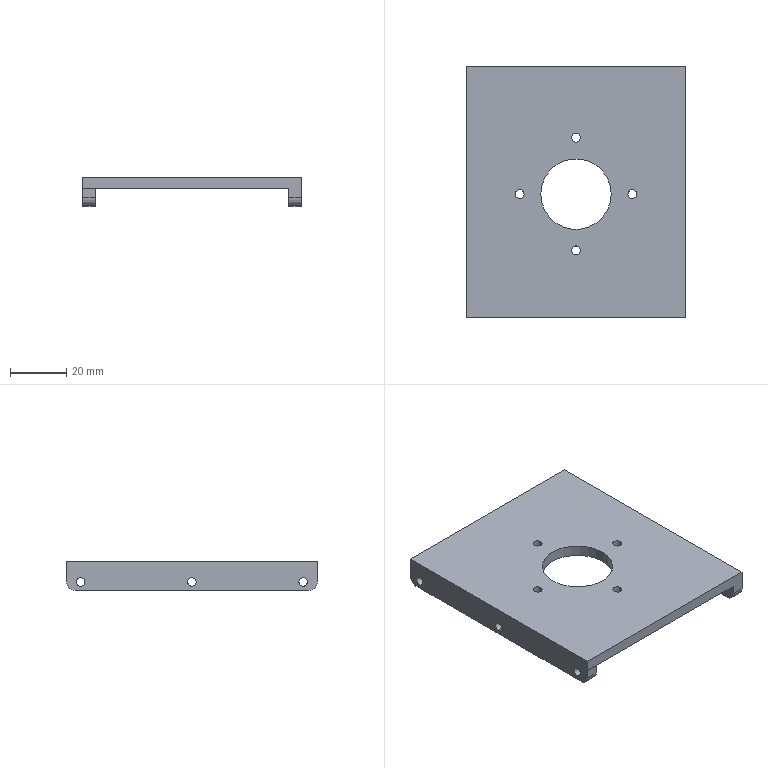Part | NX | features BREP 1 | 1 solid | 37 faces | box 77.6 x 88.919 x 10.2 mm | volume 30243 mm3 | cylinder 26 | plane 11 | commonest cylinder face diameters 3 x12 3.2 x8 6 x4 25 x2
STEP:
#1=CARTESIAN_POINT('',(1.788,32.303,2.5));
#2=VERTEX_POINT('',#1);
#3=CARTESIAN_POINT('',(-1.412,32.303,2.5));
#4=VERTEX_POINT('',#3);
#5=CARTESIAN_POINT('',(0.1876,32.303,2.5));
#6=DIRECTION('',(0.,0.,-1.));
#7=DIRECTION('',(-1.,0.,0.));
#8=AXIS2_PLACEMENT_3D('',#5,#6,#7);
#9=CIRCLE('',#8,1.6);
#10=EDGE_CURVE('',#2,#4,#9,.T.);
#11=ORIENTED_EDGE('',*,*,#10,.F.);
#12=CARTESIAN_POINT('',(1.788,32.303,-1.5));
#13=VERTEX_POINT('',#12);
#14=CARTESIAN_POINT('',(1.788,32.303,2.5));
#15=DIRECTION('',(0.,0.,-1.));
#16=VECTOR('',#15,1000.);
#17=LINE('',#14,#16);
#18=EDGE_CURVE('',#13,#2,#17,.F.);
#19=ORIENTED_EDGE('',*,*,#18,.F.);
#20=CARTESIAN_POINT('',(-1.412,32.303,-1.5));
#21=VERTEX_POINT('',#20);
#22=CARTESIAN_POINT('',(0.1876,32.303,-1.5));
#23=DIRECTION('',(0.,0.,-1.));
#24=DIRECTION('',(-1.,0.,0.));
#25=AXIS2_PLACEMENT_3D('',#22,#23,#24);
#26=CIRCLE('',#25,1.6);
#27=EDGE_CURVE('',#13,#21,#26,.T.);
#28=ORIENTED_EDGE('',*,*,#27,.T.);
#29=CARTESIAN_POINT('',(-1.412,32.303,2.5));
#30=DIRECTION('',(0.,0.,-1.));
#31=VECTOR('',#30,1000.);
#32=LINE('',#29,#31);
#33=EDGE_CURVE('',#21,#4,#32,.F.);
#34=ORIENTED_EDGE('',*,*,#33,.T.);
#35=EDGE_LOOP('',(#11,#19,#28,#34));
#36=FACE_BOUND('',#35,.T.);
#37=CARTESIAN_POINT('',(0.1876,32.303,2.5));
#38=DIRECTION('',(0.,0.,-1.));
#39=DIRECTION('',(1.,0.,0.));
#40=AXIS2_PLACEMENT_3D('',#37,#38,#39);
#41=CYLINDRICAL_SURFACE('',#40,1.6);
#42=ADVANCED_FACE('',(#36),#41,.F.);
#43=CARTESIAN_POINT('',(-18.212,52.303,2.5));
#44=VERTEX_POINT('',#43);
#45=CARTESIAN_POINT('',(-21.412,52.303,2.5));
#46=VERTEX_POINT('',#45);
#47=CARTESIAN_POINT('',(-19.812,52.303,2.5));
#48=DIRECTION('',(0.,0.,-1.));
#49=DIRECTION('',(-1.,0.,0.));
#50=AXIS2_PLACEMENT_3D('',#47,#48,#49);
#51=CIRCLE('',#50,1.6);
#52=EDGE_CURVE('',#44,#46,#51,.T.);
#53=ORIENTED_EDGE('',*,*,#52,.F.);
#54=CARTESIAN_POINT('',(-18.212,52.303,-1.5));
#55=VERTEX_POINT('',#54);
#56=CARTESIAN_POINT('',(-18.212,52.303,2.5));
#57=DIRECTION('',(0.,0.,-1.));
#58=VECTOR('',#57,1000.);
#59=LINE('',#56,#58);
#60=EDGE_CURVE('',#55,#44,#59,.F.);
#61=ORIENTED_EDGE('',*,*,#60,.F.);
#62=CARTESIAN_POINT('',(-21.412,52.303,-1.5));
#63=VERTEX_POINT('',#62);
#64=CARTESIAN_POINT('',(-19.812,52.303,-1.5));
#65=DIRECTION('',(0.,0.,-1.));
#66=DIRECTION('',(-1.,0.,0.));
#67=AXIS2_PLACEMENT_3D('',#64,#65,#66);
#68=CIRCLE('',#67,1.6);
#69=EDGE_CURVE('',#55,#63,#68,.T.);
#70=ORIENTED_EDGE('',*,*,#69,.T.);
#71=CARTESIAN_POINT('',(-21.412,52.303,2.5));
#72=DIRECTION('',(0.,0.,-1.));
#73=VECTOR('',#72,1000.);
#74=LINE('',#71,#73);
#75=EDGE_CURVE('',#63,#46,#74,.F.);
#76=ORIENTED_EDGE('',*,*,#75,.T.);
#77=EDGE_LOOP('',(#53,#61,#70,#76));
#78=FACE_BOUND('',#77,.T.);
#79=CARTESIAN_POINT('',(-19.812,52.303,2.5));
#80=DIRECTION('',(0.,0.,-1.));
#81=DIRECTION('',(1.,0.,0.));
#82=AXIS2_PLACEMENT_3D('',#79,#80,#81);
#83=CYLINDRICAL_SURFACE('',#82,1.6);
#84=ADVANCED_FACE('',(#78),#83,.F.);
#85=CARTESIAN_POINT('',(1.788,72.303,2.5));
#86=VERTEX_POINT('',#85);
#87=CARTESIAN_POINT('',(-1.412,72.303,2.5));
#88=VERTEX_POINT('',#87);
#89=CARTESIAN_POINT('',(0.1876,72.303,2.5));
#90=DIRECTION('',(0.,0.,-1.));
#91=DIRECTION('',(-1.,0.,0.));
#92=AXIS2_PLACEMENT_3D('',#89,#90,#91);
#93=CIRCLE('',#92,1.6);
#94=EDGE_CURVE('',#86,#88,#93,.T.);
#95=ORIENTED_EDGE('',*,*,#94,.F.);
#96=CARTESIAN_POINT('',(1.788,72.303,-1.5));
#97=VERTEX_POINT('',#96);
#98=CARTESIAN_POINT('',(1.788,72.303,2.5));
#99=DIRECTION('',(0.,0.,-1.));
#100=VECTOR('',#99,1000.);
#101=LINE('',#98,#100);
#102=EDGE_CURVE('',#97,#86,#101,.F.);
#103=ORIENTED_EDGE('',*,*,#102,.F.);
#104=CARTESIAN_POINT('',(-1.412,72.303,-1.5));
#105=VERTEX_POINT('',#104);
#106=CARTESIAN_POINT('',(0.1876,72.303,-1.5));
#107=DIRECTION('',(0.,0.,-1.));
#108=DIRECTION('',(-1.,0.,0.));
#109=AXIS2_PLACEMENT_3D('',#106,#107,#108);
#110=CIRCLE('',#109,1.6);
#111=EDGE_CURVE('',#97,#105,#110,.T.);
#112=ORIENTED_EDGE('',*,*,#111,.T.);
#113=CARTESIAN_POINT('',(-1.412,72.303,2.5));
#114=DIRECTION('',(0.,0.,-1.));
#115=VECTOR('',#114,1000.);
#116=LINE('',#113,#115);
#117=EDGE_CURVE('',#105,#88,#116,.F.);
#118=ORIENTED_EDGE('',*,*,#117,.T.);
#119=EDGE_LOOP('',(#95,#103,#112,#118));
#120=FACE_BOUND('',#119,.T.);
#121=CARTESIAN_POINT('',(0.1876,72.303,2.5));
#122=DIRECTION('',(0.,0.,-1.));
#123=DIRECTION('',(1.,0.,0.));
#124=AXIS2_PLACEMENT_3D('',#121,#122,#123);
#125=CYLINDRICAL_SURFACE('',#124,1.6);
#126=ADVANCED_FACE('',(#120),#125,.F.);
#127=CARTESIAN_POINT('',(21.788,52.303,2.5));
#128=VERTEX_POINT('',#127);
#129=CARTESIAN_POINT('',(18.588,52.303,2.5));
#130=VERTEX_POINT('',#129);
#131=CARTESIAN_POINT('',(20.188,52.303,2.5));
#132=DIRECTION('',(0.,0.,-1.));
#133=DIRECTION('',(-1.,0.,0.));
#134=AXIS2_PLACEMENT_3D('',#131,#132,#133);
#135=CIRCLE('',#134,1.6);
#136=EDGE_CURVE('',#128,#130,#135,.T.);
#137=ORIENTED_EDGE('',*,*,#136,.F.);
#138=CARTESIAN_POINT('',(21.788,52.303,-1.5));
#139=VERTEX_POINT('',#138);
#140=CARTESIAN_POINT('',(21.788,52.303,2.5));
#141=DIRECTION('',(0.,0.,-1.));
#142=VECTOR('',#141,1000.);
#143=LINE('',#140,#142);
#144=EDGE_CURVE('',#139,#128,#143,.F.);
#145=ORIENTED_EDGE('',*,*,#144,.F.);
#146=CARTESIAN_POINT('',(18.588,52.303,-1.5));
#147=VERTEX_POINT('',#146);
#148=CARTESIAN_POINT('',(20.188,52.303,-1.5));
#149=DIRECTION('',(0.,0.,-1.));
#150=DIRECTION('',(-1.,0.,0.));
#151=AXIS2_PLACEMENT_3D('',#148,#149,#150);
#152=CIRCLE('',#151,1.6);
#153=EDGE_CURVE('',#139,#147,#152,.T.);
#154=ORIENTED_EDGE('',*,*,#153,.T.);
#155=CARTESIAN_POINT('',(18.588,52.303,2.5));
#156=DIRECTION('',(0.,0.,-1.));
#157=VECTOR('',#156,1000.);
#158=LINE('',#155,#157);
#159=EDGE_CURVE('',#147,#130,#158,.F.);
#160=ORIENTED_EDGE('',*,*,#159,.T.);
#161=EDGE_LOOP('',(#137,#145,#154,#160));
#162=FACE_BOUND('',#161,.T.);
#163=CARTESIAN_POINT('',(20.188,52.303,2.5));
#164=DIRECTION('',(0.,0.,-1.));
#165=DIRECTION('',(1.,0.,0.));
#166=AXIS2_PLACEMENT_3D('',#163,#164,#165);
#167=CYLINDRICAL_SURFACE('',#166,1.6);
#168=ADVANCED_FACE('',(#162),#167,.F.);
#169=CARTESIAN_POINT('',(12.688,52.303,2.5));
#170=VERTEX_POINT('',#169);
#171=CARTESIAN_POINT('',(-12.312,52.303,2.5));
#172=VERTEX_POINT('',#171);
#173=CARTESIAN_POINT('',(0.1876,52.303,2.5));
#174=DIRECTION('',(0.,0.,-1.));
#175=DIRECTION('',(-1.,0.,0.));
#176=AXIS2_PLACEMENT_3D('',#173,#174,#175);
#177=CIRCLE('',#176,12.5);
#178=EDGE_CURVE('',#170,#172,#177,.T.);
#179=ORIENTED_EDGE('',*,*,#178,.F.);
#180=CARTESIAN_POINT('',(12.688,52.303,-1.5));
#181=VERTEX_POINT('',#180);
#182=CARTESIAN_POINT('',(12.688,52.303,2.5));
#183=DIRECTION('',(0.,0.,-1.));
#184=VECTOR('',#183,1000.);
#185=LINE('',#182,#184);
#186=EDGE_CURVE('',#181,#170,#185,.F.);
#187=ORIENTED_EDGE('',*,*,#186,.F.);
#188=CARTESIAN_POINT('',(-12.312,52.303,-1.5));
#189=VERTEX_POINT('',#188);
#190=CARTESIAN_POINT('',(0.1876,52.303,-1.5));
#191=DIRECTION('',(0.,0.,-1.));
#192=DIRECTION('',(-1.,0.,0.));
#193=AXIS2_PLACEMENT_3D('',#190,#191,#192);
#194=CIRCLE('',#193,12.5);
#195=EDGE_CURVE('',#181,#189,#194,.T.);
#196=ORIENTED_EDGE('',*,*,#195,.T.);
#197=CARTESIAN_POINT('',(-12.312,52.303,2.5));
#198=DIRECTION('',(0.,0.,-1.));
#199=VECTOR('',#198,1000.);
#200=LINE('',#197,#199);
#201=EDGE_CURVE('',#189,#172,#200,.F.);
#202=ORIENTED_EDGE('',*,*,#201,.T.);
#203=EDGE_LOOP('',(#179,#187,#196,#202));
#204=FACE_BOUND('',#203,.T.);
#205=CARTESIAN_POINT('',(0.1876,52.303,2.5));
#206=DIRECTION('',(0.,0.,-1.));
#207=DIRECTION('',(1.,0.,0.));
#208=AXIS2_PLACEMENT_3D('',#205,#206,#207);
#209=CYLINDRICAL_SURFACE('',#208,12.5);
#210=ADVANCED_FACE('',(#204),#209,.F.);
#211=CARTESIAN_POINT('',(38.988,92.505,-6.2));
#212=VERTEX_POINT('',#211);
#213=CARTESIAN_POINT('',(38.988,92.505,-3.2));
#214=VERTEX_POINT('',#213);
#215=CARTESIAN_POINT('',(38.988,92.505,-4.7));
#216=DIRECTION('',(-1.,0.,0.));
#217=DIRECTION('',(0.,-1.,0.));
#218=AXIS2_PLACEMENT_3D('',#215,#216,#217);
#219=CIRCLE('',#218,1.5);
#220=EDGE_CURVE('',#212,#214,#219,.T.);
#221=ORIENTED_EDGE('',*,*,#220,.F.);
#222=CARTESIAN_POINT('',(34.488,92.505,-6.2));
#223=VERTEX_POINT('',#222);
#224=CARTESIAN_POINT('',(59.388,92.505,-6.2));
#225=DIRECTION('',(-1.,0.,0.));
#226=VECTOR('',#225,1000.);
#227=LINE('',#224,#226);
#228=EDGE_CURVE('',#212,#223,#227,.T.);
#229=ORIENTED_EDGE('',*,*,#228,.T.);
#230=CARTESIAN_POINT('',(34.488,92.505,-3.2));
#231=VERTEX_POINT('',#230);
#232=CARTESIAN_POINT('',(34.488,92.505,-4.7));
#233=DIRECTION('',(1.,0.,0.));
#234=DIRECTION('',(0.,0.,-1.));
#235=AXIS2_PLACEMENT_3D('',#232,#233,#234);
#236=CIRCLE('',#235,1.5);
#237=EDGE_CURVE('',#231,#223,#236,.T.);
#238=ORIENTED_EDGE('',*,*,#237,.F.);
#239=CARTESIAN_POINT('',(59.388,92.505,-3.2));
#240=DIRECTION('',(-1.,0.,0.));
#241=VECTOR('',#240,1000.);
#242=LINE('',#239,#241);
#243=EDGE_CURVE('',#214,#231,#242,.T.);
#244=ORIENTED_EDGE('',*,*,#243,.F.);
#245=EDGE_LOOP('',(#221,#229,#238,#244));
#246=FACE_BOUND('',#245,.T.);
#247=CARTESIAN_POINT('',(59.388,92.505,-4.7));
#248=DIRECTION('',(-1.,0.,0.));
#249=DIRECTION('',(0.,0.,-1.));
#250=AXIS2_PLACEMENT_3D('',#247,#248,#249);
#251=CYLINDRICAL_SURFACE('',#250,1.5);
#252=ADVANCED_FACE('',(#246),#251,.F.);
#253=CARTESIAN_POINT('',(-34.112,92.505,-6.2));
#254=VERTEX_POINT('',#253);
#255=CARTESIAN_POINT('',(-34.112,92.505,-3.2));
#256=VERTEX_POINT('',#255);
#257=CARTESIAN_POINT('',(-34.112,92.505,-4.7));
#258=DIRECTION('',(-1.,0.,0.));
#259=DIRECTION('',(0.,0.,1.));
#260=AXIS2_PLACEMENT_3D('',#257,#258,#259);
#261=CIRCLE('',#260,1.5);
#262=EDGE_CURVE('',#254,#256,#261,.T.);
#263=ORIENTED_EDGE('',*,*,#262,.F.);
#264=CARTESIAN_POINT('',(-38.612,92.505,-6.2));
#265=VERTEX_POINT('',#264);
#266=CARTESIAN_POINT('',(-18.612,92.505,-6.2));
#267=DIRECTION('',(-1.,0.,0.));
#268=VECTOR('',#267,1000.);
#269=LINE('',#266,#268);
#270=EDGE_CURVE('',#254,#265,#269,.T.);
#271=ORIENTED_EDGE('',*,*,#270,.T.);
#272=CARTESIAN_POINT('',(-38.612,92.505,-3.2));
#273=VERTEX_POINT('',#272);
#274=CARTESIAN_POINT('',(-38.612,92.505,-4.7));
#275=DIRECTION('',(-1.,0.,0.));
#276=DIRECTION('',(0.,0.,1.));
#277=AXIS2_PLACEMENT_3D('',#274,#275,#276);
#278=CIRCLE('',#277,1.5);
#279=EDGE_CURVE('',#265,#273,#278,.T.);
#280=ORIENTED_EDGE('',*,*,#279,.T.);
#281=CARTESIAN_POINT('',(-18.612,92.505,-3.2));
#282=DIRECTION('',(-1.,0.,0.));
#283=VECTOR('',#282,1000.);
#284=LINE('',#281,#283);
#285=EDGE_CURVE('',#256,#273,#284,.T.);
#286=ORIENTED_EDGE('',*,*,#285,.F.);
#287=EDGE_LOOP('',(#263,#271,#280,#286));
#288=FACE_BOUND('',#287,.T.);
#289=CARTESIAN_POINT('',(-18.612,92.505,-4.7));
#290=DIRECTION('',(-1.,0.,0.));
#291=DIRECTION('',(0.,0.,-1.));
#292=AXIS2_PLACEMENT_3D('',#289,#290,#291);
#293=CYLINDRICAL_SURFACE('',#292,1.5);
#294=ADVANCED_FACE('',(#288),#293,.F.);
#295=CARTESIAN_POINT('',(-34.112,13.621,-6.2));
#296=VERTEX_POINT('',#295);
#297=CARTESIAN_POINT('',(-34.112,13.621,-3.2));
#298=VERTEX_POINT('',#297);
#299=CARTESIAN_POINT('',(-34.112,13.621,-4.7));
#300=DIRECTION('',(-1.,0.,0.));
#301=DIRECTION('',(0.,0.,1.));
#302=AXIS2_PLACEMENT_3D('',#299,#300,#301);
#303=CIRCLE('',#302,1.5);
#304=EDGE_CURVE('',#296,#298,#303,.T.);
#305=ORIENTED_EDGE('',*,*,#304,.F.);
#306=CARTESIAN_POINT('',(-38.612,13.621,-6.2));
#307=VERTEX_POINT('',#306);
#308=CARTESIAN_POINT('',(-18.612,13.621,-6.2));
#309=DIRECTION('',(-1.,0.,0.));
#310=VECTOR('',#309,1000.);
#311=LINE('',#308,#310);
#312=EDGE_CURVE('',#296,#307,#311,.T.);
#313=ORIENTED_EDGE('',*,*,#312,.T.);
#314=CARTESIAN_POINT('',(-38.612,13.621,-3.2));
#315=VERTEX_POINT('',#314);
#316=CARTESIAN_POINT('',(-38.612,13.621,-4.7));
#317=DIRECTION('',(-1.,0.,0.));
#318=DIRECTION('',(0.,0.,1.));
#319=AXIS2_PLACEMENT_3D('',#316,#317,#318);
#320=CIRCLE('',#319,1.5);
#321=EDGE_CURVE('',#307,#315,#320,.T.);
#322=ORIENTED_EDGE('',*,*,#321,.T.);
#323=CARTESIAN_POINT('',(-18.612,13.621,-3.2));
#324=DIRECTION('',(-1.,0.,0.));
#325=VECTOR('',#324,1000.);
#326=LINE('',#323,#325);
#327=EDGE_CURVE('',#298,#315,#326,.T.);
#328=ORIENTED_EDGE('',*,*,#327,.F.);
#329=EDGE_LOOP('',(#305,#313,#322,#328));
#330=FACE_BOUND('',#329,.T.);
#331=CARTESIAN_POINT('',(-18.612,13.621,-4.7));
#332=DIRECTION('',(-1.,0.,0.));
#333=DIRECTION('',(0.,0.,-1.));
#334=AXIS2_PLACEMENT_3D('',#331,#332,#333);
#335=CYLINDRICAL_SURFACE('',#334,1.5);
#336=ADVANCED_FACE('',(#330),#335,.F.);
#337=CARTESIAN_POINT('',(-34.112,53.063,-6.2));
#338=VERTEX_POINT('',#337);
#339=CARTESIAN_POINT('',(-34.112,53.063,-3.2));
#340=VERTEX_POINT('',#339);
#341=CARTESIAN_POINT('',(-34.112,53.063,-4.7));
#342=DIRECTION('',(-1.,0.,0.));
#343=DIRECTION('',(0.,0.,1.));
#344=AXIS2_PLACEMENT_3D('',#341,#342,#343);
#345=CIRCLE('',#344,1.5);
#346=EDGE_CURVE('',#338,#340,#345,.T.);
#347=ORIENTED_EDGE('',*,*,#346,.F.);
#348=CARTESIAN_POINT('',(-38.612,53.063,-6.2));
#349=VERTEX_POINT('',#348);
#350=CARTESIAN_POINT('',(-18.612,53.063,-6.2));
#351=DIRECTION('',(-1.,0.,0.));
#352=VECTOR('',#351,1000.);
#353=LINE('',#350,#352);
#354=EDGE_CURVE('',#338,#349,#353,.T.);
#355=ORIENTED_EDGE('',*,*,#354,.T.);
#356=CARTESIAN_POINT('',(-38.612,53.063,-3.2));
#357=VERTEX_POINT('',#356);
#358=CARTESIAN_POINT('',(-38.612,53.063,-4.7));
#359=DIRECTION('',(-1.,0.,0.));
#360=DIRECTION('',(0.,0.,1.));
#361=AXIS2_PLACEMENT_3D('',#358,#359,#360);
#362=CIRCLE('',#361,1.5);
#363=EDGE_CURVE('',#349,#357,#362,.T.);
#364=ORIENTED_EDGE('',*,*,#363,.T.);
#365=CARTESIAN_POINT('',(-18.612,53.063,-3.2));
#366=DIRECTION('',(-1.,0.,0.));
#367=VECTOR('',#366,1000.);
#368=LINE('',#365,#367);
#369=EDGE_CURVE('',#340,#357,#368,.T.);
#370=ORIENTED_EDGE('',*,*,#369,.F.);
#371=EDGE_LOOP('',(#347,#355,#364,#370));
#372=FACE_BOUND('',#371,.T.);
#373=CARTESIAN_POINT('',(-18.612,53.063,-4.7));
#374=DIRECTION('',(-1.,0.,0.));
#375=DIRECTION('',(0.,0.,-1.));
#376=AXIS2_PLACEMENT_3D('',#373,#374,#375);
#377=CYLINDRICAL_SURFACE('',#376,1.5);
#378=ADVANCED_FACE('',(#372),#377,.F.);
#379=CARTESIAN_POINT('',(34.488,12.121,-4.7));
#380=VERTEX_POINT('',#379);
#381=CARTESIAN_POINT('',(34.488,15.121,-4.7));
#382=VERTEX_POINT('',#381);
#383=CARTESIAN_POINT('',(34.488,13.621,-4.7));
#384=DIRECTION('',(1.,0.,0.));
#385=DIRECTION('',(0.,0.,-1.));
#386=AXIS2_PLACEMENT_3D('',#383,#384,#385);
#387=CIRCLE('',#386,1.5);
#388=EDGE_CURVE('',#380,#382,#387,.T.);
#389=ORIENTED_EDGE('',*,*,#388,.F.);
#390=CARTESIAN_POINT('',(38.988,12.121,-4.7));
#391=VERTEX_POINT('',#390);
#392=CARTESIAN_POINT('',(28.988,12.121,-4.7));
#393=DIRECTION('',(1.,0.,0.));
#394=VECTOR('',#393,1000.);
#395=LINE('',#392,#394);
#396=EDGE_CURVE('',#380,#391,#395,.T.);
#397=ORIENTED_EDGE('',*,*,#396,.T.);
#398=CARTESIAN_POINT('',(38.988,15.121,-4.7));
#399=VERTEX_POINT('',#398);
#400=CARTESIAN_POINT('',(38.988,13.621,-4.7));
#401=DIRECTION('',(-1.,0.,0.));
#402=DIRECTION('',(0.,-1.,0.));
#403=AXIS2_PLACEMENT_3D('',#400,#401,#402);
#404=CIRCLE('',#403,1.5);
#405=EDGE_CURVE('',#399,#391,#404,.T.);
#406=ORIENTED_EDGE('',*,*,#405,.F.);
#407=CARTESIAN_POINT('',(28.988,15.121,-4.7));
#408=DIRECTION('',(1.,0.,0.));
#409=VECTOR('',#408,1000.);
#410=LINE('',#407,#409);
#411=EDGE_CURVE('',#382,#399,#410,.T.);
#412=ORIENTED_EDGE('',*,*,#411,.F.);
#413=EDGE_LOOP('',(#389,#397,#406,#412));
#414=FACE_BOUND('',#413,.T.);
#415=CARTESIAN_POINT('',(28.988,13.621,-4.7));
#416=DIRECTION('',(1.,0.,0.));
#417=DIRECTION('',(0.,-1.,0.));
#418=AXIS2_PLACEMENT_3D('',#415,#416,#417);
#419=CYLINDRICAL_SURFACE('',#418,1.5);
#420=ADVANCED_FACE('',(#414),#419,.F.);
#421=CARTESIAN_POINT('',(34.488,51.563,-4.7));
#422=VERTEX_POINT('',#421);
#423=CARTESIAN_POINT('',(34.488,54.563,-4.7));
#424=VERTEX_POINT('',#423);
#425=CARTESIAN_POINT('',(34.488,53.063,-4.7));
#426=DIRECTION('',(1.,0.,0.));
#427=DIRECTION('',(0.,0.,-1.));
#428=AXIS2_PLACEMENT_3D('',#425,#426,#427);
#429=CIRCLE('',#428,1.5);
#430=EDGE_CURVE('',#422,#424,#429,.T.);
#431=ORIENTED_EDGE('',*,*,#430,.F.);
#432=CARTESIAN_POINT('',(38.988,51.563,-4.7));
#433=VERTEX_POINT('',#432);
#434=CARTESIAN_POINT('',(28.988,51.563,-4.7));
#435=DIRECTION('',(1.,0.,0.));
#436=VECTOR('',#435,1000.);
#437=LINE('',#434,#436);
#438=EDGE_CURVE('',#422,#433,#437,.T.);
#439=ORIENTED_EDGE('',*,*,#438,.T.);
#440=CARTESIAN_POINT('',(38.988,54.563,-4.7));
#441=VERTEX_POINT('',#440);
#442=CARTESIAN_POINT('',(38.988,53.063,-4.7));
#443=DIRECTION('',(-1.,0.,0.));
#444=DIRECTION('',(0.,-1.,0.));
#445=AXIS2_PLACEMENT_3D('',#442,#443,#444);
#446=CIRCLE('',#445,1.5);
#447=EDGE_CURVE('',#441,#433,#446,.T.);
#448=ORIENTED_EDGE('',*,*,#447,.F.);
#449=CARTESIAN_POINT('',(28.988,54.563,-4.7));
#450=DIRECTION('',(1.,0.,0.));
#451=VECTOR('',#450,1000.);
#452=LINE('',#449,#451);
#453=EDGE_CURVE('',#424,#441,#452,.T.);
#454=ORIENTED_EDGE('',*,*,#453,.F.);
#455=EDGE_LOOP('',(#431,#439,#448,#454));
#456=FACE_BOUND('',#455,.T.);
#457=CARTESIAN_POINT('',(28.988,53.063,-4.7));
#458=DIRECTION('',(1.,0.,0.));
#459=DIRECTION('',(0.,-1.,0.));
#460=AXIS2_PLACEMENT_3D('',#457,#458,#459);
#461=CYLINDRICAL_SURFACE('',#460,1.5);
#462=ADVANCED_FACE('',(#456),#461,.F.);
#463=CARTESIAN_POINT('',(38.988,97.505,-4.7));
#464=VERTEX_POINT('',#463);
#465=CARTESIAN_POINT('',(34.488,97.505,-4.7));
#466=VERTEX_POINT('',#465);
#467=CARTESIAN_POINT('',(40.988,97.505,-4.7));
#468=DIRECTION('',(-1.,0.,0.));
#469=VECTOR('',#468,1000.);
#470=LINE('',#467,#469);
#471=EDGE_CURVE('',#464,#466,#470,.T.);
#472=ORIENTED_EDGE('',*,*,#471,.F.);
#473=CARTESIAN_POINT('',(38.988,94.505,-7.7));
#474=VERTEX_POINT('',#473);
#475=CARTESIAN_POINT('',(38.988,94.505,-4.7));
#476=DIRECTION('',(-1.,0.,0.));
#477=DIRECTION('',(0.,-1.,0.));
#478=AXIS2_PLACEMENT_3D('',#475,#476,#477);
#479=CIRCLE('',#478,3.);
#480=EDGE_CURVE('',#464,#474,#479,.T.);
#481=ORIENTED_EDGE('',*,*,#480,.T.);
#482=CARTESIAN_POINT('',(34.488,94.505,-7.7));
#483=VERTEX_POINT('',#482);
#484=CARTESIAN_POINT('',(-27.612,94.505,-7.7));
#485=DIRECTION('',(1.,0.,0.));
#486=VECTOR('',#485,1000.);
#487=LINE('',#484,#486);
#488=EDGE_CURVE('',#483,#474,#487,.T.);
#489=ORIENTED_EDGE('',*,*,#488,.F.);
#490=CARTESIAN_POINT('',(34.488,94.505,-4.7));
#491=DIRECTION('',(-1.,0.,0.));
#492=DIRECTION('',(0.,0.,-1.));
#493=AXIS2_PLACEMENT_3D('',#490,#491,#492);
#494=CIRCLE('',#493,3.);
#495=EDGE_CURVE('',#466,#483,#494,.T.);
#496=ORIENTED_EDGE('',*,*,#495,.F.);
#497=EDGE_LOOP('',(#472,#481,#489,#496));
#498=FACE_BOUND('',#497,.T.);
#499=CARTESIAN_POINT('',(40.988,94.505,-4.7));
#500=DIRECTION('',(-1.,0.,0.));
#501=DIRECTION('',(0.,0.,-1.));
#502=AXIS2_PLACEMENT_3D('',#499,#500,#501);
#503=CYLINDRICAL_SURFACE('',#502,3.);
#504=ADVANCED_FACE('',(#498),#503,.T.);
#505=ORIENTED_EDGE('',*,*,#438,.F.);
#506=CARTESIAN_POINT('',(34.488,53.063,-4.7));
#507=DIRECTION('',(1.,0.,0.));
#508=DIRECTION('',(0.,0.,-1.));
#509=AXIS2_PLACEMENT_3D('',#506,#507,#508);
#510=CIRCLE('',#509,1.5);
#511=EDGE_CURVE('',#424,#422,#510,.T.);
#512=ORIENTED_EDGE('',*,*,#511,.F.);
#513=ORIENTED_EDGE('',*,*,#453,.T.);
#514=CARTESIAN_POINT('',(38.988,53.063,-4.7));
#515=DIRECTION('',(-1.,0.,0.));
#516=DIRECTION('',(0.,-1.,0.));
#517=AXIS2_PLACEMENT_3D('',#514,#515,#516);
#518=CIRCLE('',#517,1.5);
#519=EDGE_CURVE('',#433,#441,#518,.T.);
#520=ORIENTED_EDGE('',*,*,#519,.F.);
#521=EDGE_LOOP('',(#505,#512,#513,#520));
#522=FACE_BOUND('',#521,.T.);
#523=CARTESIAN_POINT('',(28.988,53.063,-4.7));
#524=DIRECTION('',(1.,0.,0.));
#525=DIRECTION('',(0.,-1.,0.));
#526=AXIS2_PLACEMENT_3D('',#523,#524,#525);
#527=CYLINDRICAL_SURFACE('',#526,1.5);
#528=ADVANCED_FACE('',(#522),#527,.F.);
#529=ORIENTED_EDGE('',*,*,#396,.F.);
#530=CARTESIAN_POINT('',(34.488,13.621,-4.7));
#531=DIRECTION('',(1.,0.,0.));
#532=DIRECTION('',(0.,0.,-1.));
#533=AXIS2_PLACEMENT_3D('',#530,#531,#532);
#534=CIRCLE('',#533,1.5);
#535=EDGE_CURVE('',#382,#380,#534,.T.);
#536=ORIENTED_EDGE('',*,*,#535,.F.);
#537=ORIENTED_EDGE('',*,*,#411,.T.);
#538=CARTESIAN_POINT('',(38.988,13.621,-4.7));
#539=DIRECTION('',(-1.,0.,0.));
#540=DIRECTION('',(0.,-1.,0.));
#541=AXIS2_PLACEMENT_3D('',#538,#539,#540);
#542=CIRCLE('',#541,1.5);
#543=EDGE_CURVE('',#391,#399,#542,.T.);
#544=ORIENTED_EDGE('',*,*,#543,.F.);
#545=EDGE_LOOP('',(#529,#536,#537,#544));
#546=FACE_BOUND('',#545,.T.);
#547=CARTESIAN_POINT('',(28.988,13.621,-4.7));
#548=DIRECTION('',(1.,0.,0.));
#549=DIRECTION('',(0.,-1.,0.));
#550=AXIS2_PLACEMENT_3D('',#547,#548,#549);
#551=CYLINDRICAL_SURFACE('',#550,1.5);
#552=ADVANCED_FACE('',(#546),#551,.F.);
#553=CARTESIAN_POINT('',(38.988,11.586,-7.7));
#554=VERTEX_POINT('',#553);
#555=CARTESIAN_POINT('',(34.488,11.586,-7.7));
#556=VERTEX_POINT('',#555);
#557=CARTESIAN_POINT('',(-27.612,11.586,-7.7));
#558=DIRECTION('',(-1.,0.,0.));
#559=VECTOR('',#558,1000.);
#560=LINE('',#557,#559);
#561=EDGE_CURVE('',#554,#556,#560,.T.);
#562=ORIENTED_EDGE('',*,*,#561,.F.);
#563=CARTESIAN_POINT('',(38.988,8.586,-4.7));
#564=VERTEX_POINT('',#563);
#565=CARTESIAN_POINT('',(38.988,11.586,-4.7));
#566=DIRECTION('',(-1.,0.,0.));
#567=DIRECTION('',(0.,-1.,0.));
#568=AXIS2_PLACEMENT_3D('',#565,#566,#567);
#569=CIRCLE('',#568,3.);
#570=EDGE_CURVE('',#554,#564,#569,.T.);
#571=ORIENTED_EDGE('',*,*,#570,.T.);
#572=CARTESIAN_POINT('',(34.488,8.586,-4.7));
#573=VERTEX_POINT('',#572);
#574=CARTESIAN_POINT('',(40.988,8.586,-4.7));
#575=DIRECTION('',(1.,0.,0.));
#576=VECTOR('',#575,1000.);
#577=LINE('',#574,#576);
#578=EDGE_CURVE('',#573,#564,#577,.T.);
#579=ORIENTED_EDGE('',*,*,#578,.F.);
#580=CARTESIAN_POINT('',(34.488,11.586,-4.7));
#581=DIRECTION('',(-1.,0.,0.));
#582=DIRECTION('',(0.,0.,-1.));
#583=AXIS2_PLACEMENT_3D('',#580,#581,#582);
#584=CIRCLE('',#583,3.);
#585=EDGE_CURVE('',#556,#573,#584,.T.);
#586=ORIENTED_EDGE('',*,*,#585,.F.);
#587=EDGE_LOOP('',(#562,#571,#579,#586));
#588=FACE_BOUND('',#587,.T.);
#589=CARTESIAN_POINT('',(40.988,11.586,-4.7));
#590=DIRECTION('',(1.,0.,0.));
#591=DIRECTION('',(0.,-1.,0.));
#592=AXIS2_PLACEMENT_3D('',#589,#590,#591);
#593=CYLINDRICAL_SURFACE('',#592,3.);
#594=ADVANCED_FACE('',(#588),#593,.T.);
#595=CARTESIAN_POINT('',(-38.612,8.586,-1.5));
#596=VERTEX_POINT('',#595);
#597=CARTESIAN_POINT('',(34.488,8.586,-1.5));
#598=VERTEX_POINT('',#597);
#599=CARTESIAN_POINT('',(40.988,8.586,-1.5));
#600=DIRECTION('',(1.,0.,0.));
#601=VECTOR('',#600,1000.);
#602=LINE('',#599,#601);
#603=EDGE_CURVE('',#596,#598,#602,.T.);
#604=ORIENTED_EDGE('',*,*,#603,.F.);
#605=CARTESIAN_POINT('',(-38.612,8.621,-1.5));
#606=VERTEX_POINT('',#605);
#607=CARTESIAN_POINT('',(-38.612,8.621,-1.5));
#608=DIRECTION('',(0.,-1.,0.));
#609=VECTOR('',#608,1000.);
#610=LINE('',#607,#609);
#611=EDGE_CURVE('',#606,#596,#610,.T.);
#612=ORIENTED_EDGE('',*,*,#611,.F.);
#613=CARTESIAN_POINT('',(-34.112,8.621,-1.5));
#614=VERTEX_POINT('',#613);
#615=CARTESIAN_POINT('',(-38.612,8.621,-1.5));
#616=DIRECTION('',(-1.,0.,0.));
#617=VECTOR('',#616,1000.);
#618=LINE('',#615,#617);
#619=EDGE_CURVE('',#614,#606,#618,.T.);
#620=ORIENTED_EDGE('',*,*,#619,.F.);
#621=CARTESIAN_POINT('',(-34.112,97.505,-1.5));
#622=VERTEX_POINT('',#621);
#623=CARTESIAN_POINT('',(-34.112,97.505,-1.5));
#624=DIRECTION('',(0.,-1.,0.));
#625=VECTOR('',#624,1000.);
#626=LINE('',#623,#625);
#627=EDGE_CURVE('',#622,#614,#626,.T.);
#628=ORIENTED_EDGE('',*,*,#627,.F.);
#629=CARTESIAN_POINT('',(34.488,97.505,-1.5));
#630=VERTEX_POINT('',#629);
#631=CARTESIAN_POINT('',(40.988,97.505,-1.5));
#632=DIRECTION('',(-1.,0.,0.));
#633=VECTOR('',#632,1000.);
#634=LINE('',#631,#633);
#635=EDGE_CURVE('',#630,#622,#634,.T.);
#636=ORIENTED_EDGE('',*,*,#635,.F.);
#637=CARTESIAN_POINT('',(34.488,8.586,-1.5));
#638=DIRECTION('',(0.,1.,0.));
#639=VECTOR('',#638,1000.);
#640=LINE('',#637,#639);
#641=EDGE_CURVE('',#598,#630,#640,.T.);
#642=ORIENTED_EDGE('',*,*,#641,.F.);
#643=EDGE_LOOP('',(#604,#612,#620,#628,#636,#642));
#644=FACE_BOUND('',#643,.T.);
#645=CARTESIAN_POINT('',(0.1876,32.303,-1.5));
#646=DIRECTION('',(0.,0.,-1.));
#647=DIRECTION('',(-1.,0.,0.));
#648=AXIS2_PLACEMENT_3D('',#645,#646,#647);
#649=CIRCLE('',#648,1.6);
#650=EDGE_CURVE('',#21,#13,#649,.T.);
#651=ORIENTED_EDGE('',*,*,#650,.F.);
#652=ORIENTED_EDGE('',*,*,#27,.F.);
#653=EDGE_LOOP('',(#651,#652));
#654=FACE_BOUND('',#653,.T.);
#655=CARTESIAN_POINT('',(-19.812,52.303,-1.5));
#656=DIRECTION('',(0.,0.,-1.));
#657=DIRECTION('',(-1.,0.,0.));
#658=AXIS2_PLACEMENT_3D('',#655,#656,#657);
#659=CIRCLE('',#658,1.6);
#660=EDGE_CURVE('',#63,#55,#659,.T.);
#661=ORIENTED_EDGE('',*,*,#660,.F.);
#662=ORIENTED_EDGE('',*,*,#69,.F.);
#663=EDGE_LOOP('',(#661,#662));
#664=FACE_BOUND('',#663,.T.);
#665=CARTESIAN_POINT('',(0.1876,72.303,-1.5));
#666=DIRECTION('',(0.,0.,-1.));
#667=DIRECTION('',(-1.,0.,0.));
#668=AXIS2_PLACEMENT_3D('',#665,#666,#667);
#669=CIRCLE('',#668,1.6);
#670=EDGE_CURVE('',#105,#97,#669,.T.);
#671=ORIENTED_EDGE('',*,*,#670,.F.);
#672=ORIENTED_EDGE('',*,*,#111,.F.);
#673=EDGE_LOOP('',(#671,#672));
#674=FACE_BOUND('',#673,.T.);
#675=CARTESIAN_POINT('',(20.188,52.303,-1.5));
#676=DIRECTION('',(0.,0.,-1.));
#677=DIRECTION('',(-1.,0.,0.));
#678=AXIS2_PLACEMENT_3D('',#675,#676,#677);
#679=CIRCLE('',#678,1.6);
#680=EDGE_CURVE('',#147,#139,#679,.T.);
#681=ORIENTED_EDGE('',*,*,#680,.F.);
#682=ORIENTED_EDGE('',*,*,#153,.F.);
#683=EDGE_LOOP('',(#681,#682));
#684=FACE_BOUND('',#683,.T.);
#685=CARTESIAN_POINT('',(0.1876,52.303,-1.5));
#686=DIRECTION('',(0.,0.,-1.));
#687=DIRECTION('',(-1.,0.,0.));
#688=AXIS2_PLACEMENT_3D('',#685,#686,#687);
#689=CIRCLE('',#688,12.5);
#690=EDGE_CURVE('',#189,#181,#689,.T.);
#691=ORIENTED_EDGE('',*,*,#690,.F.);
#692=ORIENTED_EDGE('',*,*,#195,.F.);
#693=EDGE_LOOP('',(#691,#692));
#694=FACE_BOUND('',#693,.T.);
#695=CARTESIAN_POINT('',(0.,0.,-1.5));
#696=DIRECTION('',(0.,0.,1.));
#697=DIRECTION('',(-1.,0.,0.));
#698=AXIS2_PLACEMENT_3D('',#695,#696,#697);
#699=PLANE('',#698);
#700=ADVANCED_FACE('',(#644,#654,#664,#674,#684,#694),#699,.F.);
#701=ORIENTED_EDGE('',*,*,#619,.T.);
#702=CARTESIAN_POINT('',(-38.612,8.621,-4.7));
#703=VERTEX_POINT('',#702);
#704=CARTESIAN_POINT('',(-38.612,8.621,-4.7));
#705=DIRECTION('',(0.,0.,1.));
#706=VECTOR('',#705,1000.);
#707=LINE('',#704,#706);
#708=EDGE_CURVE('',#703,#606,#707,.T.);
#709=ORIENTED_EDGE('',*,*,#708,.F.);
#710=CARTESIAN_POINT('',(-34.112,8.621,-4.7));
#711=VERTEX_POINT('',#710);
#712=CARTESIAN_POINT('',(-38.612,8.621,-4.7));
#713=DIRECTION('',(1.,0.,0.));
#714=VECTOR('',#713,1000.);
#715=LINE('',#712,#714);
#716=EDGE_CURVE('',#703,#711,#715,.T.);
#717=ORIENTED_EDGE('',*,*,#716,.T.);
#718=CARTESIAN_POINT('',(-34.112,8.621,-95.698));
#719=DIRECTION('',(0.,0.,1.));
#720=VECTOR('',#719,1000.);
#721=LINE('',#718,#720);
#722=EDGE_CURVE('',#711,#614,#721,.T.);
#723=ORIENTED_EDGE('',*,*,#722,.T.);
#724=EDGE_LOOP('',(#701,#709,#717,#723));
#725=FACE_BOUND('',#724,.T.);
#726=CARTESIAN_POINT('',(-38.612,8.621,-95.698));
#727=DIRECTION('',(0.,1.,0.));
#728=DIRECTION('',(-1.,0.,0.));
#729=AXIS2_PLACEMENT_3D('',#726,#727,#728);
#730=PLANE('',#729);
#731=ADVANCED_FACE('',(#725),#730,.F.);
#732=ORIENTED_EDGE('',*,*,#354,.F.);
#733=CARTESIAN_POINT('',(-34.112,53.063,-4.7));
#734=DIRECTION('',(-1.,0.,0.));
#735=DIRECTION('',(0.,0.,1.));
#736=AXIS2_PLACEMENT_3D('',#733,#734,#735);
#737=CIRCLE('',#736,1.5);
#738=EDGE_CURVE('',#340,#338,#737,.T.);
#739=ORIENTED_EDGE('',*,*,#738,.F.);
#740=ORIENTED_EDGE('',*,*,#369,.T.);
#741=CARTESIAN_POINT('',(-38.612,53.063,-4.7));
#742=DIRECTION('',(-1.,0.,0.));
#743=DIRECTION('',(0.,0.,1.));
#744=AXIS2_PLACEMENT_3D('',#741,#742,#743);
#745=CIRCLE('',#744,1.5);
#746=EDGE_CURVE('',#357,#349,#745,.T.);
#747=ORIENTED_EDGE('',*,*,#746,.T.);
#748=EDGE_LOOP('',(#732,#739,#740,#747));
#749=FACE_BOUND('',#748,.T.);
#750=CARTESIAN_POINT('',(-18.612,53.063,-4.7));
#751=DIRECTION('',(-1.,0.,0.));
#752=DIRECTION('',(0.,0.,-1.));
#753=AXIS2_PLACEMENT_3D('',#750,#751,#752);
#754=CYLINDRICAL_SURFACE('',#753,1.5);
#755=ADVANCED_FACE('',(#749),#754,.F.);
#756=ORIENTED_EDGE('',*,*,#312,.F.);
#757=CARTESIAN_POINT('',(-34.112,13.621,-4.7));
#758=DIRECTION('',(-1.,0.,0.));
#759=DIRECTION('',(0.,0.,1.));
#760=AXIS2_PLACEMENT_3D('',#757,#758,#759);
#761=CIRCLE('',#760,1.5);
#762=EDGE_CURVE('',#298,#296,#761,.T.);
#763=ORIENTED_EDGE('',*,*,#762,.F.);
#764=ORIENTED_EDGE('',*,*,#327,.T.);
#765=CARTESIAN_POINT('',(-38.612,13.621,-4.7));
#766=DIRECTION('',(-1.,0.,0.));
#767=DIRECTION('',(0.,0.,1.));
#768=AXIS2_PLACEMENT_3D('',#765,#766,#767);
#769=CIRCLE('',#768,1.5);
#770=EDGE_CURVE('',#315,#307,#769,.T.);
#771=ORIENTED_EDGE('',*,*,#770,.T.);
#772=EDGE_LOOP('',(#756,#763,#764,#771));
#773=FACE_BOUND('',#772,.T.);
#774=CARTESIAN_POINT('',(-18.612,13.621,-4.7));
#775=DIRECTION('',(-1.,0.,0.));
#776=DIRECTION('',(0.,0.,-1.));
#777=AXIS2_PLACEMENT_3D('',#774,#775,#776);
#778=CYLINDRICAL_SURFACE('',#777,1.5);
#779=ADVANCED_FACE('',(#773),#778,.F.);
#780=ORIENTED_EDGE('',*,*,#716,.F.);
#781=CARTESIAN_POINT('',(-38.612,11.621,-7.7));
#782=VERTEX_POINT('',#781);
#783=CARTESIAN_POINT('',(-38.612,11.621,-4.7));
#784=DIRECTION('',(-1.,0.,0.));
#785=DIRECTION('',(0.,0.,1.));
#786=AXIS2_PLACEMENT_3D('',#783,#784,#785);
#787=CIRCLE('',#786,3.);
#788=EDGE_CURVE('',#782,#703,#787,.T.);
#789=ORIENTED_EDGE('',*,*,#788,.F.);
#790=CARTESIAN_POINT('',(-34.112,11.621,-7.7));
#791=VERTEX_POINT('',#790);
#792=CARTESIAN_POINT('',(-27.612,11.621,-7.7));
#793=DIRECTION('',(-1.,0.,0.));
#794=VECTOR('',#793,1000.);
#795=LINE('',#792,#794);
#796=EDGE_CURVE('',#791,#782,#795,.T.);
#797=ORIENTED_EDGE('',*,*,#796,.F.);
#798=CARTESIAN_POINT('',(-34.112,11.621,-4.7));
#799=DIRECTION('',(1.,0.,0.));
#800=DIRECTION('',(0.,0.,1.));
#801=AXIS2_PLACEMENT_3D('',#798,#799,#800);
#802=CIRCLE('',#801,3.);
#803=EDGE_CURVE('',#711,#791,#802,.T.);
#804=ORIENTED_EDGE('',*,*,#803,.F.);
#805=EDGE_LOOP('',(#780,#789,#797,#804));
#806=FACE_BOUND('',#805,.T.);
#807=CARTESIAN_POINT('',(-38.612,11.621,-4.7));
#808=DIRECTION('',(1.,0.,0.));
#809=DIRECTION('',(0.,0.,1.));
#810=AXIS2_PLACEMENT_3D('',#807,#808,#809);
#811=CYLINDRICAL_SURFACE('',#810,3.);
#812=ADVANCED_FACE('',(#806),#811,.T.);
#813=ORIENTED_EDGE('',*,*,#570,.F.);
#814=CARTESIAN_POINT('',(38.988,17.621,-7.7));
#815=VERTEX_POINT('',#814);
#816=CARTESIAN_POINT('',(38.988,11.621,-7.7));
#817=DIRECTION('',(0.,-1.,-0.000000247));
#818=VECTOR('',#817,1000.);
#819=LINE('',#816,#818);
#820=EDGE_CURVE('',#554,#815,#819,.F.);
#821=ORIENTED_EDGE('',*,*,#820,.T.);
#822=CARTESIAN_POINT('',(38.988,49.063,-7.7));
#823=VERTEX_POINT('',#822);
#824=CARTESIAN_POINT('',(38.988,8.586,-7.7));
#825=DIRECTION('',(0.,1.,0.000000494));
#826=VECTOR('',#825,1000.);
#827=LINE('',#824,#826);
#828=EDGE_CURVE('',#815,#823,#827,.T.);
#829=ORIENTED_EDGE('',*,*,#828,.T.);
#830=CARTESIAN_POINT('',(38.988,57.063,-7.7));
#831=VERTEX_POINT('',#830);
#832=CARTESIAN_POINT('',(38.988,49.063,-7.7));
#833=DIRECTION('',(0.,-1.,-0.000000247));
#834=VECTOR('',#833,1000.);
#835=LINE('',#832,#834);
#836=EDGE_CURVE('',#831,#823,#835,.T.);
#837=ORIENTED_EDGE('',*,*,#836,.F.);
#838=CARTESIAN_POINT('',(38.988,88.505,-7.7));
#839=VERTEX_POINT('',#838);
#840=CARTESIAN_POINT('',(38.988,8.586,-7.7));
#841=DIRECTION('',(0.,1.,0.000000494));
#842=VECTOR('',#841,1000.);
#843=LINE('',#840,#842);
#844=EDGE_CURVE('',#839,#831,#843,.F.);
#845=ORIENTED_EDGE('',*,*,#844,.F.);
#846=CARTESIAN_POINT('',(38.988,88.505,-7.7));
#847=DIRECTION('',(0.,-1.,-0.000000247));
#848=VECTOR('',#847,1000.);
#849=LINE('',#846,#848);
#850=EDGE_CURVE('',#474,#839,#849,.T.);
#851=ORIENTED_EDGE('',*,*,#850,.F.);
#852=ORIENTED_EDGE('',*,*,#480,.F.);
#853=CARTESIAN_POINT('',(38.988,97.505,2.5));
#854=VERTEX_POINT('',#853);
#855=CARTESIAN_POINT('',(38.988,97.505,3.));
#856=DIRECTION('',(0.,0.,1.));
#857=VECTOR('',#856,1000.);
#858=LINE('',#855,#857);
#859=EDGE_CURVE('',#464,#854,#858,.T.);
#860=ORIENTED_EDGE('',*,*,#859,.T.);
#861=CARTESIAN_POINT('',(38.988,8.586,2.5));
#862=VERTEX_POINT('',#861);
#863=CARTESIAN_POINT('',(38.988,8.586,2.5));
#864=DIRECTION('',(0.,1.,0.));
#865=VECTOR('',#864,1000.);
#866=LINE('',#863,#865);
#867=EDGE_CURVE('',#862,#854,#866,.T.);
#868=ORIENTED_EDGE('',*,*,#867,.F.);
#869=CARTESIAN_POINT('',(38.988,8.586,3.));
#870=DIRECTION('',(0.,0.,-1.));
#871=VECTOR('',#870,1000.);
#872=LINE('',#869,#871);
#873=EDGE_CURVE('',#862,#564,#872,.T.);
#874=ORIENTED_EDGE('',*,*,#873,.T.);
#875=EDGE_LOOP('',(#813,#821,#829,#837,#845,#851,#852,#860,#868,#874));
#876=FACE_BOUND('',#875,.T.);
#877=ORIENTED_EDGE('',*,*,#447,.T.);
#878=ORIENTED_EDGE('',*,*,#519,.T.);
#879=EDGE_LOOP('',(#877,#878));
#880=FACE_BOUND('',#879,.T.);
#881=CARTESIAN_POINT('',(38.988,92.505,-4.7));
#882=DIRECTION('',(-1.,0.,0.));
#883=DIRECTION('',(0.,-1.,0.));
#884=AXIS2_PLACEMENT_3D('',#881,#882,#883);
#885=CIRCLE('',#884,1.5);
#886=EDGE_CURVE('',#214,#212,#885,.T.);
#887=ORIENTED_EDGE('',*,*,#886,.T.);
#888=ORIENTED_EDGE('',*,*,#220,.T.);
#889=EDGE_LOOP('',(#887,#888));
#890=FACE_BOUND('',#889,.T.);
#891=ORIENTED_EDGE('',*,*,#405,.T.);
#892=ORIENTED_EDGE('',*,*,#543,.T.);
#893=EDGE_LOOP('',(#891,#892));
#894=FACE_BOUND('',#893,.T.);
#895=CARTESIAN_POINT('',(38.988,8.586,3.));
#896=DIRECTION('',(-1.,0.,0.));
#897=DIRECTION('',(0.,-1.,0.));
#898=AXIS2_PLACEMENT_3D('',#895,#896,#897);
#899=PLANE('',#898);
#900=ADVANCED_FACE('',(#876,#880,#890,#894),#899,.F.);
#901=ORIENTED_EDGE('',*,*,#859,.F.);
#902=ORIENTED_EDGE('',*,*,#471,.T.);
#903=CARTESIAN_POINT('',(34.488,97.505,-96.733));
#904=DIRECTION('',(0.,0.,1.));
#905=VECTOR('',#904,1000.);
#906=LINE('',#903,#905);
#907=EDGE_CURVE('',#466,#630,#906,.T.);
#908=ORIENTED_EDGE('',*,*,#907,.T.);
#909=ORIENTED_EDGE('',*,*,#635,.T.);
#910=CARTESIAN_POINT('',(-34.112,97.505,-4.7));
#911=VERTEX_POINT('',#910);
#912=CARTESIAN_POINT('',(-34.112,97.505,-95.698));
#913=DIRECTION('',(0.,0.,1.));
#914=VECTOR('',#913,1000.);
#915=LINE('',#912,#914);
#916=EDGE_CURVE('',#911,#622,#915,.T.);
#917=ORIENTED_EDGE('',*,*,#916,.F.);
#918=CARTESIAN_POINT('',(-38.612,97.505,-4.7));
#919=VERTEX_POINT('',#918);
#920=CARTESIAN_POINT('',(40.988,97.505,-4.7));
#921=DIRECTION('',(-1.,0.,0.));
#922=VECTOR('',#921,1000.);
#923=LINE('',#920,#922);
#924=EDGE_CURVE('',#911,#919,#923,.T.);
#925=ORIENTED_EDGE('',*,*,#924,.T.);
#926=CARTESIAN_POINT('',(-38.612,97.505,2.5));
#927=VERTEX_POINT('',#926);
#928=CARTESIAN_POINT('',(-38.612,97.505,-2.049));
#929=DIRECTION('',(0.,0.,1.));
#930=VECTOR('',#929,1000.);
#931=LINE('',#928,#930);
#932=EDGE_CURVE('',#919,#927,#931,.T.);
#933=ORIENTED_EDGE('',*,*,#932,.T.);
#934=CARTESIAN_POINT('',(40.988,97.505,2.5));
#935=DIRECTION('',(-1.,0.,0.));
#936=VECTOR('',#935,1000.);
#937=LINE('',#934,#936);
#938=EDGE_CURVE('',#854,#927,#937,.T.);
#939=ORIENTED_EDGE('',*,*,#938,.F.);
#940=EDGE_LOOP('',(#901,#902,#908,#909,#917,#925,#933,#939));
#941=FACE_BOUND('',#940,.T.);
#942=CARTESIAN_POINT('',(40.988,97.505,3.));
#943=DIRECTION('',(0.,-1.,0.));
#944=DIRECTION('',(0.,0.,1.));
#945=AXIS2_PLACEMENT_3D('',#942,#943,#944);
#946=PLANE('',#945);
#947=ADVANCED_FACE('',(#941),#946,.F.);
#948=ORIENTED_EDGE('',*,*,#578,.T.);
#949=ORIENTED_EDGE('',*,*,#873,.F.);
#950=CARTESIAN_POINT('',(-38.612,8.586,2.5));
#951=VERTEX_POINT('',#950);
#952=CARTESIAN_POINT('',(40.988,8.586,2.5));
#953=DIRECTION('',(1.,0.,0.));
#954=VECTOR('',#953,1000.);
#955=LINE('',#952,#954);
#956=EDGE_CURVE('',#951,#862,#955,.T.);
#957=ORIENTED_EDGE('',*,*,#956,.F.);
#958=CARTESIAN_POINT('',(-38.612,8.586,3.));
#959=DIRECTION('',(0.,0.,1.));
#960=VECTOR('',#959,1000.);
#961=LINE('',#958,#960);
#962=EDGE_CURVE('',#596,#951,#961,.T.);
#963=ORIENTED_EDGE('',*,*,#962,.F.);
#964=ORIENTED_EDGE('',*,*,#603,.T.);
#965=CARTESIAN_POINT('',(34.488,8.586,-96.733));
#966=DIRECTION('',(0.,0.,1.));
#967=VECTOR('',#966,1000.);
#968=LINE('',#965,#967);
#969=EDGE_CURVE('',#573,#598,#968,.T.);
#970=ORIENTED_EDGE('',*,*,#969,.F.);
#971=EDGE_LOOP('',(#948,#949,#957,#963,#964,#970));
#972=FACE_BOUND('',#971,.T.);
#973=CARTESIAN_POINT('',(40.988,8.586,3.));
#974=DIRECTION('',(0.,1.,0.));
#975=DIRECTION('',(-1.,0.,0.));
#976=AXIS2_PLACEMENT_3D('',#973,#974,#975);
#977=PLANE('',#976);
#978=ADVANCED_FACE('',(#972),#977,.F.);
#979=ORIENTED_EDGE('',*,*,#956,.T.);
#980=ORIENTED_EDGE('',*,*,#867,.T.);
#981=ORIENTED_EDGE('',*,*,#938,.T.);
#982=CARTESIAN_POINT('',(-38.612,0.,2.5));
#983=DIRECTION('',(0.,1.,0.));
#984=VECTOR('',#983,1000.);
#985=LINE('',#982,#984);
#986=EDGE_CURVE('',#951,#927,#985,.T.);
#987=ORIENTED_EDGE('',*,*,#986,.F.);
#988=EDGE_LOOP('',(#979,#980,#981,#987));
#989=FACE_BOUND('',#988,.T.);
#990=CARTESIAN_POINT('',(0.1876,32.303,2.5));
#991=DIRECTION('',(0.,0.,-1.));
#992=DIRECTION('',(-1.,0.,0.));
#993=AXIS2_PLACEMENT_3D('',#990,#991,#992);
#994=CIRCLE('',#993,1.6);
#995=EDGE_CURVE('',#4,#2,#994,.T.);
#996=ORIENTED_EDGE('',*,*,#995,.T.);
#997=ORIENTED_EDGE('',*,*,#10,.T.);
#998=EDGE_LOOP('',(#996,#997));
#999=FACE_BOUND('',#998,.T.);
#1000=CARTESIAN_POINT('',(-19.812,52.303,2.5));
#1001=DIRECTION('',(0.,0.,-1.));
#1002=DIRECTION('',(-1.,0.,0.));
#1003=AXIS2_PLACEMENT_3D('',#1000,#1001,#1002);
#1004=CIRCLE('',#1003,1.6);
#1005=EDGE_CURVE('',#46,#44,#1004,.T.);
#1006=ORIENTED_EDGE('',*,*,#1005,.T.);
#1007=ORIENTED_EDGE('',*,*,#52,.T.);
#1008=EDGE_LOOP('',(#1006,#1007));
#1009=FACE_BOUND('',#1008,.T.);
#1010=CARTESIAN_POINT('',(0.1876,72.303,2.5));
#1011=DIRECTION('',(0.,0.,-1.));
#1012=DIRECTION('',(-1.,0.,0.));
#1013=AXIS2_PLACEMENT_3D('',#1010,#1011,#1012);
#1014=CIRCLE('',#1013,1.6);
#1015=EDGE_CURVE('',#88,#86,#1014,.T.);
#1016=ORIENTED_EDGE('',*,*,#1015,.T.);
#1017=ORIENTED_EDGE('',*,*,#94,.T.);
#1018=EDGE_LOOP('',(#1016,#1017));
#1019=FACE_BOUND('',#1018,.T.);
#1020=CARTESIAN_POINT('',(20.188,52.303,2.5));
#1021=DIRECTION('',(0.,0.,-1.));
#1022=DIRECTION('',(-1.,0.,0.));
#1023=AXIS2_PLACEMENT_3D('',#1020,#1021,#1022);
#1024=CIRCLE('',#1023,1.6);
#1025=EDGE_CURVE('',#130,#128,#1024,.T.);
#1026=ORIENTED_EDGE('',*,*,#1025,.T.);
#1027=ORIENTED_EDGE('',*,*,#136,.T.);
#1028=EDGE_LOOP('',(#1026,#1027));
#1029=FACE_BOUND('',#1028,.T.);
#1030=CARTESIAN_POINT('',(0.1876,52.303,2.5));
#1031=DIRECTION('',(0.,0.,-1.));
#1032=DIRECTION('',(-1.,0.,0.));
#1033=AXIS2_PLACEMENT_3D('',#1030,#1031,#1032);
#1034=CIRCLE('',#1033,12.5);
#1035=EDGE_CURVE('',#172,#170,#1034,.T.);
#1036=ORIENTED_EDGE('',*,*,#1035,.T.);
#1037=ORIENTED_EDGE('',*,*,#178,.T.);
#1038=EDGE_LOOP('',(#1036,#1037));
#1039=FACE_BOUND('',#1038,.T.);
#1040=CARTESIAN_POINT('',(0.,0.,2.5));
#1041=DIRECTION('',(0.,0.,1.));
#1042=DIRECTION('',(-1.,0.,0.));
#1043=AXIS2_PLACEMENT_3D('',#1040,#1041,#1042);
#1044=PLANE('',#1043);
#1045=ADVANCED_FACE('',(#989,#999,#1009,#1019,#1029,#1039),#1044,.T.);
#1046=CARTESIAN_POINT('',(-38.612,49.063,-7.7));
#1047=VERTEX_POINT('',#1046);
#1048=CARTESIAN_POINT('',(-38.612,17.621,-7.7));
#1049=VERTEX_POINT('',#1048);
#1050=CARTESIAN_POINT('',(-38.612,18.212,-7.7));
#1051=DIRECTION('',(0.,-1.,-0.000000494));
#1052=VECTOR('',#1051,1000.);
#1053=LINE('',#1050,#1052);
#1054=EDGE_CURVE('',#1047,#1049,#1053,.T.);
#1055=ORIENTED_EDGE('',*,*,#1054,.T.);
#1056=CARTESIAN_POINT('',(-38.612,17.621,-7.7));
#1057=DIRECTION('',(0.,-1.,-0.000000247));
#1058=VECTOR('',#1057,1000.);
#1059=LINE('',#1056,#1058);
#1060=EDGE_CURVE('',#1049,#782,#1059,.T.);
#1061=ORIENTED_EDGE('',*,*,#1060,.T.);
#1062=ORIENTED_EDGE('',*,*,#788,.T.);
#1063=ORIENTED_EDGE('',*,*,#708,.T.);
#1064=ORIENTED_EDGE('',*,*,#611,.T.);
#1065=ORIENTED_EDGE('',*,*,#962,.T.);
#1066=ORIENTED_EDGE('',*,*,#986,.T.);
#1067=ORIENTED_EDGE('',*,*,#932,.F.);
#1068=CARTESIAN_POINT('',(-38.612,94.505,-7.7));
#1069=VERTEX_POINT('',#1068);
#1070=CARTESIAN_POINT('',(-38.612,94.505,-4.7));
#1071=DIRECTION('',(-1.,0.,0.));
#1072=DIRECTION('',(0.,0.,1.));
#1073=AXIS2_PLACEMENT_3D('',#1070,#1071,#1072);
#1074=CIRCLE('',#1073,3.);
#1075=EDGE_CURVE('',#919,#1069,#1074,.T.);
#1076=ORIENTED_EDGE('',*,*,#1075,.T.);
#1077=CARTESIAN_POINT('',(-38.612,88.505,-7.7));
#1078=VERTEX_POINT('',#1077);
#1079=CARTESIAN_POINT('',(-38.612,94.505,-7.7));
#1080=DIRECTION('',(0.,-1.,-0.000000247));
#1081=VECTOR('',#1080,1000.);
#1082=LINE('',#1079,#1081);
#1083=EDGE_CURVE('',#1069,#1078,#1082,.T.);
#1084=ORIENTED_EDGE('',*,*,#1083,.T.);
#1085=CARTESIAN_POINT('',(-38.612,57.063,-7.7));
#1086=VERTEX_POINT('',#1085);
#1087=CARTESIAN_POINT('',(-38.612,18.212,-7.7));
#1088=DIRECTION('',(0.,-1.,-0.000000494));
#1089=VECTOR('',#1088,1000.);
#1090=LINE('',#1087,#1089);
#1091=EDGE_CURVE('',#1078,#1086,#1090,.T.);
#1092=ORIENTED_EDGE('',*,*,#1091,.T.);
#1093=CARTESIAN_POINT('',(-38.612,57.063,-7.7));
#1094=DIRECTION('',(0.,-1.,-0.000000247));
#1095=VECTOR('',#1094,1000.);
#1096=LINE('',#1093,#1095);
#1097=EDGE_CURVE('',#1086,#1047,#1096,.T.);
#1098=ORIENTED_EDGE('',*,*,#1097,.T.);
#1099=EDGE_LOOP('',(#1055,#1061,#1062,#1063,#1064,#1065,#1066,#1067,#1076,#1084,#1092,#1098));
#1100=FACE_BOUND('',#1099,.T.);
#1101=ORIENTED_EDGE('',*,*,#746,.F.);
#1102=ORIENTED_EDGE('',*,*,#363,.F.);
#1103=EDGE_LOOP('',(#1101,#1102));
#1104=FACE_BOUND('',#1103,.T.);
#1105=CARTESIAN_POINT('',(-38.612,92.505,-4.7));
#1106=DIRECTION('',(-1.,0.,0.));
#1107=DIRECTION('',(0.,0.,1.));
#1108=AXIS2_PLACEMENT_3D('',#1105,#1106,#1107);
#1109=CIRCLE('',#1108,1.5);
#1110=EDGE_CURVE('',#273,#265,#1109,.T.);
#1111=ORIENTED_EDGE('',*,*,#1110,.F.);
#1112=ORIENTED_EDGE('',*,*,#279,.F.);
#1113=EDGE_LOOP('',(#1111,#1112));
#1114=FACE_BOUND('',#1113,.T.);
#1115=ORIENTED_EDGE('',*,*,#770,.F.);
#1116=ORIENTED_EDGE('',*,*,#321,.F.);
#1117=EDGE_LOOP('',(#1115,#1116));
#1118=FACE_BOUND('',#1117,.T.);
#1119=CARTESIAN_POINT('',(-38.612,0.,-2.049));
#1120=DIRECTION('',(-1.,0.,0.));
#1121=DIRECTION('',(0.,0.,-1.));
#1122=AXIS2_PLACEMENT_3D('',#1119,#1120,#1121);
#1123=PLANE('',#1122);
#1124=ADVANCED_FACE('',(#1100,#1104,#1114,#1118),#1123,.T.);
#1125=CARTESIAN_POINT('',(-34.112,94.505,-7.7));
#1126=VERTEX_POINT('',#1125);
#1127=CARTESIAN_POINT('',(-34.112,97.505,-7.7));
#1128=DIRECTION('',(0.,1.,0.000000494));
#1129=VECTOR('',#1128,1000.);
#1130=LINE('',#1127,#1129);
#1131=EDGE_CURVE('',#791,#1126,#1130,.T.);
#1132=ORIENTED_EDGE('',*,*,#1131,.T.);
#1133=CARTESIAN_POINT('',(-34.112,94.505,-4.7));
#1134=DIRECTION('',(1.,0.,0.));
#1135=DIRECTION('',(0.,0.,1.));
#1136=AXIS2_PLACEMENT_3D('',#1133,#1134,#1135);
#1137=CIRCLE('',#1136,3.);
#1138=EDGE_CURVE('',#1126,#911,#1137,.T.);
#1139=ORIENTED_EDGE('',*,*,#1138,.T.);
#1140=ORIENTED_EDGE('',*,*,#916,.T.);
#1141=ORIENTED_EDGE('',*,*,#627,.T.);
#1142=ORIENTED_EDGE('',*,*,#722,.F.);
#1143=ORIENTED_EDGE('',*,*,#803,.T.);
#1144=EDGE_LOOP('',(#1132,#1139,#1140,#1141,#1142,#1143));
#1145=FACE_BOUND('',#1144,.T.);
#1146=ORIENTED_EDGE('',*,*,#762,.T.);
#1147=ORIENTED_EDGE('',*,*,#304,.T.);
#1148=EDGE_LOOP('',(#1146,#1147));
#1149=FACE_BOUND('',#1148,.T.);
#1150=CARTESIAN_POINT('',(-34.112,92.505,-4.7));
#1151=DIRECTION('',(-1.,0.,0.));
#1152=DIRECTION('',(0.,0.,1.));
#1153=AXIS2_PLACEMENT_3D('',#1150,#1151,#1152);
#1154=CIRCLE('',#1153,1.5);
#1155=EDGE_CURVE('',#256,#254,#1154,.T.);
#1156=ORIENTED_EDGE('',*,*,#1155,.T.);
#1157=ORIENTED_EDGE('',*,*,#262,.T.);
#1158=EDGE_LOOP('',(#1156,#1157));
#1159=FACE_BOUND('',#1158,.T.);
#1160=ORIENTED_EDGE('',*,*,#738,.T.);
#1161=ORIENTED_EDGE('',*,*,#346,.T.);
#1162=EDGE_LOOP('',(#1160,#1161));
#1163=FACE_BOUND('',#1162,.T.);
#1164=CARTESIAN_POINT('',(-34.112,97.505,-95.698));
#1165=DIRECTION('',(-1.,0.,0.));
#1166=DIRECTION('',(0.,0.,-1.));
#1167=AXIS2_PLACEMENT_3D('',#1164,#1165,#1166);
#1168=PLANE('',#1167);
#1169=ADVANCED_FACE('',(#1145,#1149,#1159,#1163),#1168,.F.);
#1170=ORIENTED_EDGE('',*,*,#1060,.F.);
#1171=ORIENTED_EDGE('',*,*,#1054,.F.);
#1172=ORIENTED_EDGE('',*,*,#1097,.F.);
#1173=ORIENTED_EDGE('',*,*,#1091,.F.);
#1174=ORIENTED_EDGE('',*,*,#1083,.F.);
#1175=CARTESIAN_POINT('',(-27.612,94.505,-7.7));
#1176=DIRECTION('',(1.,0.,0.));
#1177=VECTOR('',#1176,1000.);
#1178=LINE('',#1175,#1177);
#1179=EDGE_CURVE('',#1069,#1126,#1178,.T.);
#1180=ORIENTED_EDGE('',*,*,#1179,.T.);
#1181=ORIENTED_EDGE('',*,*,#1131,.F.);
#1182=ORIENTED_EDGE('',*,*,#796,.T.);
#1183=EDGE_LOOP('',(#1170,#1171,#1172,#1173,#1174,#1180,#1181,#1182));
#1184=FACE_BOUND('',#1183,.T.);
#1185=CARTESIAN_POINT('',(-27.612,18.212,-7.7));
#1186=DIRECTION('',(0.,-0.000000494,1.));
#1187=DIRECTION('',(1.,0.,0.));
#1188=AXIS2_PLACEMENT_3D('',#1185,#1186,#1187);
#1189=PLANE('',#1188);
#1190=ADVANCED_FACE('',(#1184),#1189,.F.);
#1191=ORIENTED_EDGE('',*,*,#270,.F.);
#1192=ORIENTED_EDGE('',*,*,#1155,.F.);
#1193=ORIENTED_EDGE('',*,*,#285,.T.);
#1194=ORIENTED_EDGE('',*,*,#1110,.T.);
#1195=EDGE_LOOP('',(#1191,#1192,#1193,#1194));
#1196=FACE_BOUND('',#1195,.T.);
#1197=CARTESIAN_POINT('',(-18.612,92.505,-4.7));
#1198=DIRECTION('',(-1.,0.,0.));
#1199=DIRECTION('',(0.,0.,-1.));
#1200=AXIS2_PLACEMENT_3D('',#1197,#1198,#1199);
#1201=CYLINDRICAL_SURFACE('',#1200,1.5);
#1202=ADVANCED_FACE('',(#1196),#1201,.F.);
#1203=ORIENTED_EDGE('',*,*,#907,.F.);
#1204=ORIENTED_EDGE('',*,*,#495,.T.);
#1205=CARTESIAN_POINT('',(34.488,8.586,-7.7));
#1206=DIRECTION('',(0.,-1.,-0.000000494));
#1207=VECTOR('',#1206,1000.);
#1208=LINE('',#1205,#1207);
#1209=EDGE_CURVE('',#483,#556,#1208,.T.);
#1210=ORIENTED_EDGE('',*,*,#1209,.T.);
#1211=ORIENTED_EDGE('',*,*,#585,.T.);
#1212=ORIENTED_EDGE('',*,*,#969,.T.);
#1213=ORIENTED_EDGE('',*,*,#641,.T.);
#1214=EDGE_LOOP('',(#1203,#1204,#1210,#1211,#1212,#1213));
#1215=FACE_BOUND('',#1214,.T.);
#1216=ORIENTED_EDGE('',*,*,#237,.T.);
#1217=CARTESIAN_POINT('',(34.488,92.505,-4.7));
#1218=DIRECTION('',(1.,0.,0.));
#1219=DIRECTION('',(0.,0.,-1.));
#1220=AXIS2_PLACEMENT_3D('',#1217,#1218,#1219);
#1221=CIRCLE('',#1220,1.5);
#1222=EDGE_CURVE('',#223,#231,#1221,.T.);
#1223=ORIENTED_EDGE('',*,*,#1222,.T.);
#1224=EDGE_LOOP('',(#1216,#1223));
#1225=FACE_BOUND('',#1224,.T.);
#1226=ORIENTED_EDGE('',*,*,#535,.T.);
#1227=ORIENTED_EDGE('',*,*,#388,.T.);
#1228=EDGE_LOOP('',(#1226,#1227));
#1229=FACE_BOUND('',#1228,.T.);
#1230=ORIENTED_EDGE('',*,*,#511,.T.);
#1231=ORIENTED_EDGE('',*,*,#430,.T.);
#1232=EDGE_LOOP('',(#1230,#1231));
#1233=FACE_BOUND('',#1232,.T.);
#1234=CARTESIAN_POINT('',(34.488,8.586,-96.733));
#1235=DIRECTION('',(1.,0.,0.));
#1236=DIRECTION('',(0.,-1.,0.));
#1237=AXIS2_PLACEMENT_3D('',#1234,#1235,#1236);
#1238=PLANE('',#1237);
#1239=ADVANCED_FACE('',(#1215,#1225,#1229,#1233),#1238,.F.);
#1240=ORIENTED_EDGE('',*,*,#850,.T.);
#1241=ORIENTED_EDGE('',*,*,#844,.T.);
#1242=ORIENTED_EDGE('',*,*,#836,.T.);
#1243=ORIENTED_EDGE('',*,*,#828,.F.);
#1244=ORIENTED_EDGE('',*,*,#820,.F.);
#1245=ORIENTED_EDGE('',*,*,#561,.T.);
#1246=ORIENTED_EDGE('',*,*,#1209,.F.);
#1247=ORIENTED_EDGE('',*,*,#488,.T.);
#1248=EDGE_LOOP('',(#1240,#1241,#1242,#1243,#1244,#1245,#1246,#1247));
#1249=FACE_BOUND('',#1248,.T.);
#1250=CARTESIAN_POINT('',(-27.612,18.212,-7.7));
#1251=DIRECTION('',(0.,-0.000000494,1.));
#1252=DIRECTION('',(1.,0.,0.));
#1253=AXIS2_PLACEMENT_3D('',#1250,#1251,#1252);
#1254=PLANE('',#1253);
#1255=ADVANCED_FACE('',(#1249),#1254,.F.);
#1256=ORIENTED_EDGE('',*,*,#1179,.F.);
#1257=ORIENTED_EDGE('',*,*,#1075,.F.);
#1258=ORIENTED_EDGE('',*,*,#924,.F.);
#1259=ORIENTED_EDGE('',*,*,#1138,.F.);
#1260=EDGE_LOOP('',(#1256,#1257,#1258,#1259));
#1261=FACE_BOUND('',#1260,.T.);
#1262=CARTESIAN_POINT('',(40.988,94.505,-4.7));
#1263=DIRECTION('',(-1.,0.,0.));
#1264=DIRECTION('',(0.,0.,-1.));
#1265=AXIS2_PLACEMENT_3D('',#1262,#1263,#1264);
#1266=CYLINDRICAL_SURFACE('',#1265,3.);
#1267=ADVANCED_FACE('',(#1261),#1266,.T.);
#1268=ORIENTED_EDGE('',*,*,#228,.F.);
#1269=ORIENTED_EDGE('',*,*,#886,.F.);
#1270=ORIENTED_EDGE('',*,*,#243,.T.);
#1271=ORIENTED_EDGE('',*,*,#1222,.F.);
#1272=EDGE_LOOP('',(#1268,#1269,#1270,#1271));
#1273=FACE_BOUND('',#1272,.T.);
#1274=CARTESIAN_POINT('',(59.388,92.505,-4.7));
#1275=DIRECTION('',(-1.,0.,0.));
#1276=DIRECTION('',(0.,0.,-1.));
#1277=AXIS2_PLACEMENT_3D('',#1274,#1275,#1276);
#1278=CYLINDRICAL_SURFACE('',#1277,1.5);
#1279=ADVANCED_FACE('',(#1273),#1278,.F.);
#1280=ORIENTED_EDGE('',*,*,#186,.T.);
#1281=ORIENTED_EDGE('',*,*,#1035,.F.);
#1282=ORIENTED_EDGE('',*,*,#201,.F.);
#1283=ORIENTED_EDGE('',*,*,#690,.T.);
#1284=EDGE_LOOP('',(#1280,#1281,#1282,#1283));
#1285=FACE_BOUND('',#1284,.T.);
#1286=CARTESIAN_POINT('',(0.1876,52.303,2.5));
#1287=DIRECTION('',(0.,0.,-1.));
#1288=DIRECTION('',(1.,0.,0.));
#1289=AXIS2_PLACEMENT_3D('',#1286,#1287,#1288);
#1290=CYLINDRICAL_SURFACE('',#1289,12.5);
#1291=ADVANCED_FACE('',(#1285),#1290,.F.);
#1292=ORIENTED_EDGE('',*,*,#144,.T.);
#1293=ORIENTED_EDGE('',*,*,#1025,.F.);
#1294=ORIENTED_EDGE('',*,*,#159,.F.);
#1295=ORIENTED_EDGE('',*,*,#680,.T.);
#1296=EDGE_LOOP('',(#1292,#1293,#1294,#1295));
#1297=FACE_BOUND('',#1296,.T.);
#1298=CARTESIAN_POINT('',(20.188,52.303,2.5));
#1299=DIRECTION('',(0.,0.,-1.));
#1300=DIRECTION('',(1.,0.,0.));
#1301=AXIS2_PLACEMENT_3D('',#1298,#1299,#1300);
#1302=CYLINDRICAL_SURFACE('',#1301,1.6);
#1303=ADVANCED_FACE('',(#1297),#1302,.F.);
#1304=ORIENTED_EDGE('',*,*,#102,.T.);
#1305=ORIENTED_EDGE('',*,*,#1015,.F.);
#1306=ORIENTED_EDGE('',*,*,#117,.F.);
#1307=ORIENTED_EDGE('',*,*,#670,.T.);
#1308=EDGE_LOOP('',(#1304,#1305,#1306,#1307));
#1309=FACE_BOUND('',#1308,.T.);
#1310=CARTESIAN_POINT('',(0.1876,72.303,2.5));
#1311=DIRECTION('',(0.,0.,-1.));
#1312=DIRECTION('',(1.,0.,0.));
#1313=AXIS2_PLACEMENT_3D('',#1310,#1311,#1312);
#1314=CYLINDRICAL_SURFACE('',#1313,1.6);
#1315=ADVANCED_FACE('',(#1309),#1314,.F.);
#1316=ORIENTED_EDGE('',*,*,#60,.T.);
#1317=ORIENTED_EDGE('',*,*,#1005,.F.);
#1318=ORIENTED_EDGE('',*,*,#75,.F.);
#1319=ORIENTED_EDGE('',*,*,#660,.T.);
#1320=EDGE_LOOP('',(#1316,#1317,#1318,#1319));
#1321=FACE_BOUND('',#1320,.T.);
#1322=CARTESIAN_POINT('',(-19.812,52.303,2.5));
#1323=DIRECTION('',(0.,0.,-1.));
#1324=DIRECTION('',(1.,0.,0.));
#1325=AXIS2_PLACEMENT_3D('',#1322,#1323,#1324);
#1326=CYLINDRICAL_SURFACE('',#1325,1.6);
#1327=ADVANCED_FACE('',(#1321),#1326,.F.);
#1328=ORIENTED_EDGE('',*,*,#18,.T.);
#1329=ORIENTED_EDGE('',*,*,#995,.F.);
#1330=ORIENTED_EDGE('',*,*,#33,.F.);
#1331=ORIENTED_EDGE('',*,*,#650,.T.);
#1332=EDGE_LOOP('',(#1328,#1329,#1330,#1331));
#1333=FACE_BOUND('',#1332,.T.);
#1334=CARTESIAN_POINT('',(0.1876,32.303,2.5));
#1335=DIRECTION('',(0.,0.,-1.));
#1336=DIRECTION('',(1.,0.,0.));
#1337=AXIS2_PLACEMENT_3D('',#1334,#1335,#1336);
#1338=CYLINDRICAL_SURFACE('',#1337,1.6);
#1339=ADVANCED_FACE('',(#1333),#1338,.F.);
#1340=CLOSED_SHELL('',(#42,#84,#126,#168,#210,#252,#294,#336,#378,#420,#462,#504,#528,#552,#594,#700,#731,#755,#779,#812,#900,#947,#978,#1045,#1124,#1169,#1190,#1202,#1239,#1255,#1267,#1279,#1291,#1303,#1315,#1327,#1339));
#1341=MANIFOLD_SOLID_BREP('',#1340);
#1342=(LENGTH_UNIT()NAMED_UNIT(*)SI_UNIT(.MILLI.,.METRE.));
#1343=UNCERTAINTY_MEASURE_WITH_UNIT(LENGTH_MEASURE(0.00001),#1342,'','');
#1344=(NAMED_UNIT(*)PLANE_ANGLE_UNIT()SI_UNIT($,.RADIAN.));
#1345=(NAMED_UNIT(*)SI_UNIT($,.STERADIAN.)SOLID_ANGLE_UNIT());
#1346=(GEOMETRIC_REPRESENTATION_CONTEXT(3)GLOBAL_UNCERTAINTY_ASSIGNED_CONTEXT((#1343))GLOBAL_UNIT_ASSIGNED_CONTEXT((#1342,#1344,#1345))REPRESENTATION_CONTEXT('',''));
#1347=ADVANCED_BREP_SHAPE_REPRESENTATION('',(#1341),#1346);